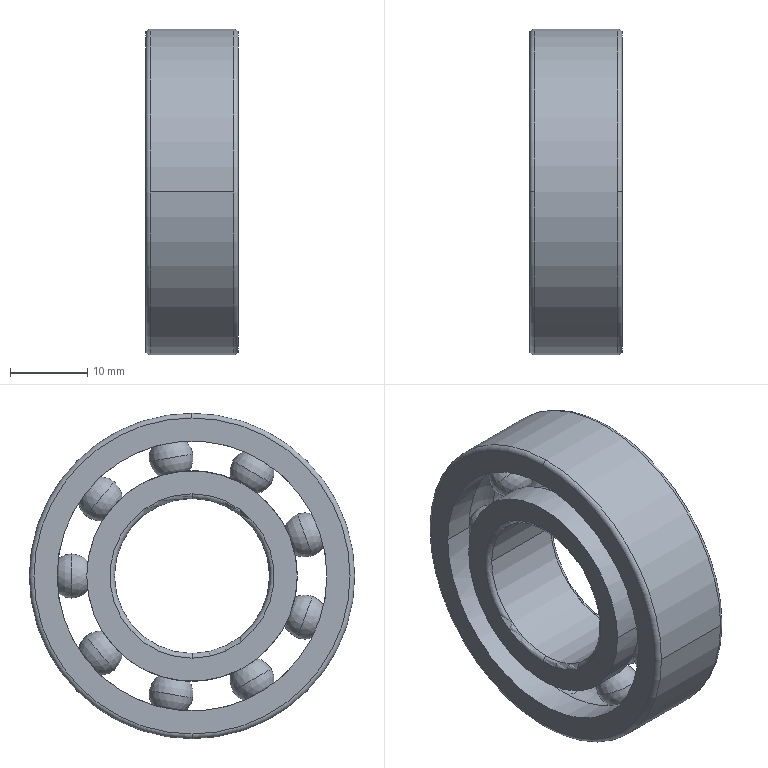Part | STEP file | KS B 2023 - 6004 - 20 x 42 x 12 | 11 solids | 75 faces | box 12 x 42 x 42 mm | volume 8691 mm3 | torus 41 | sphere 18 | cylinder 12 | plane 4 | commonest cylinder face diameters 27.172 x4 34.828 x4 20 x2 42 x2